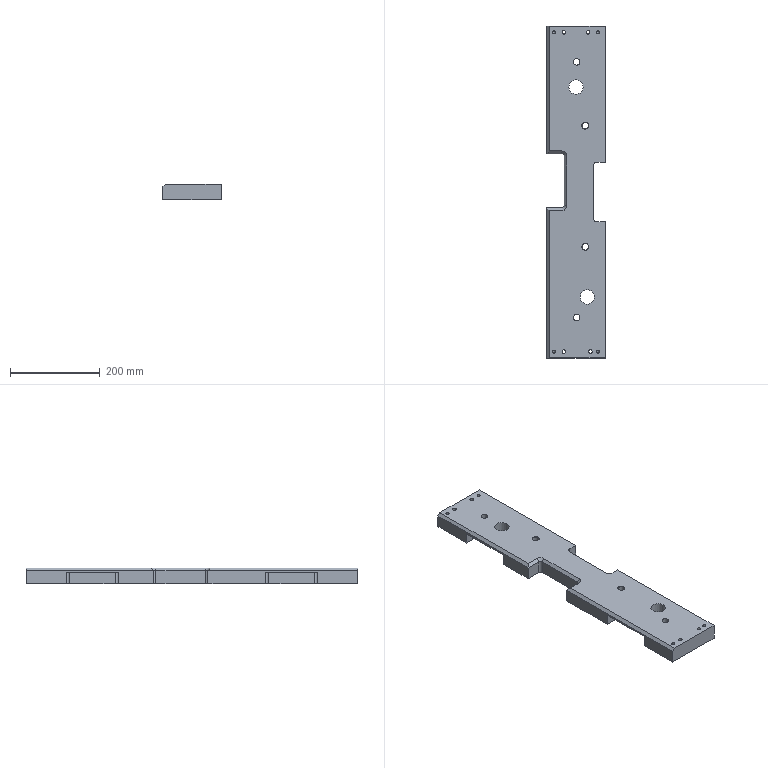Part | STEP file | lll_id4790_x_t | 1 solid | 69 faces | box 130 x 739 x 35 mm | volume 2775296 mm3 | plane 29 | cylinder 28 | cone 12 | commonest cylinder face diameters 6.806 x8 10 x6 8 x4 14 x2 14.506 x2 16 x2